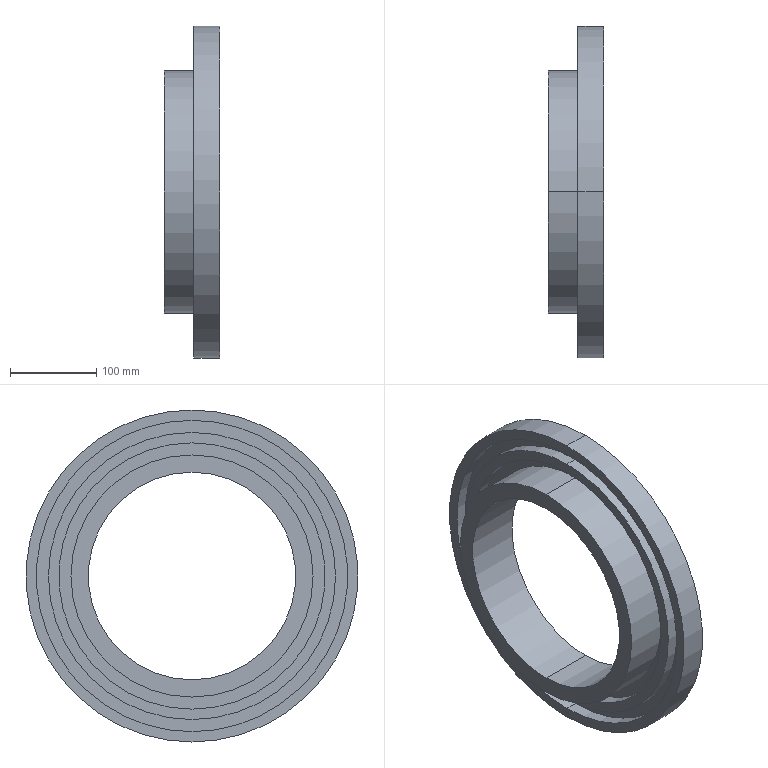Part | SolidWorks | features Revolution 1 | 1 solid | 18 faces | box 64 x 384 x 384 mm | volume 2278534 mm3 | cylinder 12 | plane 6 | commonest cylinder face diameters 240 x2 280 x2 308 x2 332 x2 360 x2 384 x2
STEP:
#1=CARTESIAN_POINT('',(64.,0.,-120.));
#2=VERTEX_POINT('',#1);
#3=CARTESIAN_POINT('',(64.,0.,120.));
#4=VERTEX_POINT('',#3);
#5=CARTESIAN_POINT('',(64.,0.,0.));
#6=DIRECTION('',(-1.,0.,0.));
#7=DIRECTION('',(0.,0.,1.));
#8=AXIS2_PLACEMENT_3D('',#5,#6,#7);
#9=CIRCLE('',#8,120.);
#10=EDGE_CURVE('',#2,#4,#9,.T.);
#11=ORIENTED_EDGE('',*,*,#10,.F.);
#12=CARTESIAN_POINT('',(0.,0.,-120.));
#13=VERTEX_POINT('',#12);
#14=CARTESIAN_POINT('',(0.,0.,-120.));
#15=DIRECTION('',(-1.,0.,0.));
#16=VECTOR('',#15,1000.);
#17=LINE('',#14,#16);
#18=EDGE_CURVE('',#2,#13,#17,.T.);
#19=ORIENTED_EDGE('',*,*,#18,.T.);
#20=CARTESIAN_POINT('',(0.,0.,120.));
#21=VERTEX_POINT('',#20);
#22=CARTESIAN_POINT('',(0.,0.,0.));
#23=DIRECTION('',(-1.,0.,0.));
#24=DIRECTION('',(0.,0.,1.));
#25=AXIS2_PLACEMENT_3D('',#22,#23,#24);
#26=CIRCLE('',#25,120.);
#27=EDGE_CURVE('',#13,#21,#26,.T.);
#28=ORIENTED_EDGE('',*,*,#27,.T.);
#29=CARTESIAN_POINT('',(0.,0.,120.));
#30=DIRECTION('',(-1.,0.,0.));
#31=VECTOR('',#30,1000.);
#32=LINE('',#29,#31);
#33=EDGE_CURVE('',#4,#21,#32,.T.);
#34=ORIENTED_EDGE('',*,*,#33,.F.);
#35=EDGE_LOOP('',(#11,#19,#28,#34));
#36=FACE_OUTER_BOUND('',#35,.T.);
#37=CARTESIAN_POINT('',(0.,0.,0.));
#38=DIRECTION('',(-1.,0.,0.));
#39=DIRECTION('',(0.,0.,1.));
#40=AXIS2_PLACEMENT_3D('',#37,#38,#39);
#41=CYLINDRICAL_SURFACE('',#40,120.);
#42=ADVANCED_FACE('',(#36),#41,.F.);
#43=CARTESIAN_POINT('',(64.,0.,192.));
#44=VERTEX_POINT('',#43);
#45=CARTESIAN_POINT('',(64.,0.,-192.));
#46=VERTEX_POINT('',#45);
#47=CARTESIAN_POINT('',(64.,0.,0.));
#48=DIRECTION('',(-1.,0.,0.));
#49=DIRECTION('',(0.,0.,1.));
#50=AXIS2_PLACEMENT_3D('',#47,#48,#49);
#51=CIRCLE('',#50,192.);
#52=EDGE_CURVE('',#44,#46,#51,.T.);
#53=ORIENTED_EDGE('',*,*,#52,.T.);
#54=CARTESIAN_POINT('',(34.,0.,-192.));
#55=VERTEX_POINT('',#54);
#56=CARTESIAN_POINT('',(0.,0.,-192.));
#57=DIRECTION('',(-1.,0.,0.));
#58=VECTOR('',#57,1000.);
#59=LINE('',#56,#58);
#60=EDGE_CURVE('',#46,#55,#59,.T.);
#61=ORIENTED_EDGE('',*,*,#60,.T.);
#62=CARTESIAN_POINT('',(34.,0.,192.));
#63=VERTEX_POINT('',#62);
#64=CARTESIAN_POINT('',(34.,0.,0.));
#65=DIRECTION('',(-1.,0.,0.));
#66=DIRECTION('',(0.,0.,1.));
#67=AXIS2_PLACEMENT_3D('',#64,#65,#66);
#68=CIRCLE('',#67,192.);
#69=EDGE_CURVE('',#63,#55,#68,.T.);
#70=ORIENTED_EDGE('',*,*,#69,.F.);
#71=CARTESIAN_POINT('',(0.,0.,192.));
#72=DIRECTION('',(-1.,0.,0.));
#73=VECTOR('',#72,1000.);
#74=LINE('',#71,#73);
#75=EDGE_CURVE('',#44,#63,#74,.T.);
#76=ORIENTED_EDGE('',*,*,#75,.F.);
#77=EDGE_LOOP('',(#53,#61,#70,#76));
#78=FACE_OUTER_BOUND('',#77,.T.);
#79=CARTESIAN_POINT('',(0.,0.,0.));
#80=DIRECTION('',(-1.,0.,0.));
#81=DIRECTION('',(0.,0.,1.));
#82=AXIS2_PLACEMENT_3D('',#79,#80,#81);
#83=CYLINDRICAL_SURFACE('',#82,192.);
#84=ADVANCED_FACE('',(#78),#83,.T.);
#85=CARTESIAN_POINT('',(48.,0.,-180.));
#86=VERTEX_POINT('',#85);
#87=CARTESIAN_POINT('',(48.,0.,180.));
#88=VERTEX_POINT('',#87);
#89=CARTESIAN_POINT('',(48.,0.,0.));
#90=DIRECTION('',(-1.,0.,0.));
#91=DIRECTION('',(0.,0.,1.));
#92=AXIS2_PLACEMENT_3D('',#89,#90,#91);
#93=CIRCLE('',#92,180.);
#94=EDGE_CURVE('',#86,#88,#93,.T.);
#95=ORIENTED_EDGE('',*,*,#94,.F.);
#96=CARTESIAN_POINT('',(34.,0.,-180.));
#97=VERTEX_POINT('',#96);
#98=CARTESIAN_POINT('',(0.,0.,-180.));
#99=DIRECTION('',(-1.,0.,0.));
#100=VECTOR('',#99,1000.);
#101=LINE('',#98,#100);
#102=EDGE_CURVE('',#86,#97,#101,.T.);
#103=ORIENTED_EDGE('',*,*,#102,.T.);
#104=CARTESIAN_POINT('',(34.,0.,180.));
#105=VERTEX_POINT('',#104);
#106=CARTESIAN_POINT('',(34.,0.,0.));
#107=DIRECTION('',(-1.,0.,0.));
#108=DIRECTION('',(0.,0.,1.));
#109=AXIS2_PLACEMENT_3D('',#106,#107,#108);
#110=CIRCLE('',#109,180.);
#111=EDGE_CURVE('',#97,#105,#110,.T.);
#112=ORIENTED_EDGE('',*,*,#111,.T.);
#113=CARTESIAN_POINT('',(0.,0.,180.));
#114=DIRECTION('',(-1.,0.,0.));
#115=VECTOR('',#114,1000.);
#116=LINE('',#113,#115);
#117=EDGE_CURVE('',#88,#105,#116,.T.);
#118=ORIENTED_EDGE('',*,*,#117,.F.);
#119=EDGE_LOOP('',(#95,#103,#112,#118));
#120=FACE_OUTER_BOUND('',#119,.T.);
#121=CARTESIAN_POINT('',(0.,0.,0.));
#122=DIRECTION('',(-1.,0.,0.));
#123=DIRECTION('',(0.,0.,1.));
#124=AXIS2_PLACEMENT_3D('',#121,#122,#123);
#125=CYLINDRICAL_SURFACE('',#124,180.);
#126=ADVANCED_FACE('',(#120),#125,.F.);
#127=CARTESIAN_POINT('',(48.,0.,166.));
#128=VERTEX_POINT('',#127);
#129=CARTESIAN_POINT('',(48.,0.,-166.));
#130=VERTEX_POINT('',#129);
#131=CARTESIAN_POINT('',(48.,0.,0.));
#132=DIRECTION('',(-1.,0.,0.));
#133=DIRECTION('',(0.,0.,1.));
#134=AXIS2_PLACEMENT_3D('',#131,#132,#133);
#135=CIRCLE('',#134,166.);
#136=EDGE_CURVE('',#128,#130,#135,.T.);
#137=ORIENTED_EDGE('',*,*,#136,.T.);
#138=CARTESIAN_POINT('',(34.,0.,-166.));
#139=VERTEX_POINT('',#138);
#140=CARTESIAN_POINT('',(0.,0.,-166.));
#141=DIRECTION('',(-1.,0.,0.));
#142=VECTOR('',#141,1000.);
#143=LINE('',#140,#142);
#144=EDGE_CURVE('',#130,#139,#143,.T.);
#145=ORIENTED_EDGE('',*,*,#144,.T.);
#146=CARTESIAN_POINT('',(34.,0.,166.));
#147=VERTEX_POINT('',#146);
#148=CARTESIAN_POINT('',(34.,0.,0.));
#149=DIRECTION('',(-1.,0.,0.));
#150=DIRECTION('',(0.,0.,1.));
#151=AXIS2_PLACEMENT_3D('',#148,#149,#150);
#152=CIRCLE('',#151,166.);
#153=EDGE_CURVE('',#147,#139,#152,.T.);
#154=ORIENTED_EDGE('',*,*,#153,.F.);
#155=CARTESIAN_POINT('',(0.,0.,166.));
#156=DIRECTION('',(-1.,0.,0.));
#157=VECTOR('',#156,1000.);
#158=LINE('',#155,#157);
#159=EDGE_CURVE('',#128,#147,#158,.T.);
#160=ORIENTED_EDGE('',*,*,#159,.F.);
#161=EDGE_LOOP('',(#137,#145,#154,#160));
#162=FACE_OUTER_BOUND('',#161,.T.);
#163=CARTESIAN_POINT('',(0.,0.,0.));
#164=DIRECTION('',(-1.,0.,0.));
#165=DIRECTION('',(0.,0.,1.));
#166=AXIS2_PLACEMENT_3D('',#163,#164,#165);
#167=CYLINDRICAL_SURFACE('',#166,166.);
#168=ADVANCED_FACE('',(#162),#167,.T.);
#169=CARTESIAN_POINT('',(48.,0.,-154.));
#170=VERTEX_POINT('',#169);
#171=CARTESIAN_POINT('',(48.,0.,154.));
#172=VERTEX_POINT('',#171);
#173=CARTESIAN_POINT('',(48.,0.,0.));
#174=DIRECTION('',(-1.,0.,0.));
#175=DIRECTION('',(0.,0.,1.));
#176=AXIS2_PLACEMENT_3D('',#173,#174,#175);
#177=CIRCLE('',#176,154.);
#178=EDGE_CURVE('',#170,#172,#177,.T.);
#179=ORIENTED_EDGE('',*,*,#178,.F.);
#180=CARTESIAN_POINT('',(34.,0.,-154.));
#181=VERTEX_POINT('',#180);
#182=CARTESIAN_POINT('',(0.,0.,-154.));
#183=DIRECTION('',(-1.,0.,0.));
#184=VECTOR('',#183,1000.);
#185=LINE('',#182,#184);
#186=EDGE_CURVE('',#170,#181,#185,.T.);
#187=ORIENTED_EDGE('',*,*,#186,.T.);
#188=CARTESIAN_POINT('',(34.,0.,154.));
#189=VERTEX_POINT('',#188);
#190=CARTESIAN_POINT('',(34.,0.,0.));
#191=DIRECTION('',(-1.,0.,0.));
#192=DIRECTION('',(0.,0.,1.));
#193=AXIS2_PLACEMENT_3D('',#190,#191,#192);
#194=CIRCLE('',#193,154.);
#195=EDGE_CURVE('',#181,#189,#194,.T.);
#196=ORIENTED_EDGE('',*,*,#195,.T.);
#197=CARTESIAN_POINT('',(0.,0.,154.));
#198=DIRECTION('',(-1.,0.,0.));
#199=VECTOR('',#198,1000.);
#200=LINE('',#197,#199);
#201=EDGE_CURVE('',#172,#189,#200,.T.);
#202=ORIENTED_EDGE('',*,*,#201,.F.);
#203=EDGE_LOOP('',(#179,#187,#196,#202));
#204=FACE_OUTER_BOUND('',#203,.T.);
#205=CARTESIAN_POINT('',(0.,0.,0.));
#206=DIRECTION('',(-1.,0.,0.));
#207=DIRECTION('',(0.,0.,1.));
#208=AXIS2_PLACEMENT_3D('',#205,#206,#207);
#209=CYLINDRICAL_SURFACE('',#208,154.);
#210=ADVANCED_FACE('',(#204),#209,.F.);
#211=CARTESIAN_POINT('',(48.,0.,140.));
#212=VERTEX_POINT('',#211);
#213=CARTESIAN_POINT('',(48.,0.,-140.));
#214=VERTEX_POINT('',#213);
#215=CARTESIAN_POINT('',(48.,0.,0.));
#216=DIRECTION('',(-1.,0.,0.));
#217=DIRECTION('',(0.,0.,1.));
#218=AXIS2_PLACEMENT_3D('',#215,#216,#217);
#219=CIRCLE('',#218,140.);
#220=EDGE_CURVE('',#212,#214,#219,.T.);
#221=ORIENTED_EDGE('',*,*,#220,.T.);
#222=CARTESIAN_POINT('',(0.,0.,-140.));
#223=VERTEX_POINT('',#222);
#224=CARTESIAN_POINT('',(0.,0.,-140.));
#225=DIRECTION('',(-1.,0.,0.));
#226=VECTOR('',#225,1000.);
#227=LINE('',#224,#226);
#228=EDGE_CURVE('',#214,#223,#227,.T.);
#229=ORIENTED_EDGE('',*,*,#228,.T.);
#230=CARTESIAN_POINT('',(0.,0.,140.));
#231=VERTEX_POINT('',#230);
#232=CARTESIAN_POINT('',(0.,0.,0.));
#233=DIRECTION('',(-1.,0.,0.));
#234=DIRECTION('',(0.,0.,1.));
#235=AXIS2_PLACEMENT_3D('',#232,#233,#234);
#236=CIRCLE('',#235,140.);
#237=EDGE_CURVE('',#231,#223,#236,.T.);
#238=ORIENTED_EDGE('',*,*,#237,.F.);
#239=CARTESIAN_POINT('',(0.,0.,140.));
#240=DIRECTION('',(-1.,0.,0.));
#241=VECTOR('',#240,1000.);
#242=LINE('',#239,#241);
#243=EDGE_CURVE('',#212,#231,#242,.T.);
#244=ORIENTED_EDGE('',*,*,#243,.F.);
#245=EDGE_LOOP('',(#221,#229,#238,#244));
#246=FACE_OUTER_BOUND('',#245,.T.);
#247=CARTESIAN_POINT('',(0.,0.,0.));
#248=DIRECTION('',(-1.,0.,0.));
#249=DIRECTION('',(0.,0.,1.));
#250=AXIS2_PLACEMENT_3D('',#247,#248,#249);
#251=CYLINDRICAL_SURFACE('',#250,140.);
#252=ADVANCED_FACE('',(#246),#251,.T.);
#253=ORIENTED_EDGE('',*,*,#228,.F.);
#254=CARTESIAN_POINT('',(48.,0.,0.));
#255=DIRECTION('',(-1.,0.,0.));
#256=DIRECTION('',(0.,0.,1.));
#257=AXIS2_PLACEMENT_3D('',#254,#255,#256);
#258=CIRCLE('',#257,140.);
#259=EDGE_CURVE('',#214,#212,#258,.T.);
#260=ORIENTED_EDGE('',*,*,#259,.T.);
#261=ORIENTED_EDGE('',*,*,#243,.T.);
#262=CARTESIAN_POINT('',(0.,0.,0.));
#263=DIRECTION('',(-1.,0.,0.));
#264=DIRECTION('',(0.,0.,1.));
#265=AXIS2_PLACEMENT_3D('',#262,#263,#264);
#266=CIRCLE('',#265,140.);
#267=EDGE_CURVE('',#223,#231,#266,.T.);
#268=ORIENTED_EDGE('',*,*,#267,.F.);
#269=EDGE_LOOP('',(#253,#260,#261,#268));
#270=FACE_OUTER_BOUND('',#269,.T.);
#271=CARTESIAN_POINT('',(0.,0.,0.));
#272=DIRECTION('',(-1.,0.,0.));
#273=DIRECTION('',(0.,0.,1.));
#274=AXIS2_PLACEMENT_3D('',#271,#272,#273);
#275=CYLINDRICAL_SURFACE('',#274,140.);
#276=ADVANCED_FACE('',(#270),#275,.T.);
#277=ORIENTED_EDGE('',*,*,#220,.F.);
#278=ORIENTED_EDGE('',*,*,#259,.F.);
#279=EDGE_LOOP('',(#277,#278));
#280=FACE_BOUND('',#279,.T.);
#281=CARTESIAN_POINT('',(48.,0.,0.));
#282=DIRECTION('',(-1.,0.,0.));
#283=DIRECTION('',(0.,0.,1.));
#284=AXIS2_PLACEMENT_3D('',#281,#282,#283);
#285=CIRCLE('',#284,154.);
#286=EDGE_CURVE('',#172,#170,#285,.T.);
#287=ORIENTED_EDGE('',*,*,#286,.T.);
#288=ORIENTED_EDGE('',*,*,#178,.T.);
#289=EDGE_LOOP('',(#287,#288));
#290=FACE_OUTER_BOUND('',#289,.T.);
#291=CARTESIAN_POINT('',(48.,154.,0.));
#292=DIRECTION('',(1.,0.,0.));
#293=DIRECTION('',(0.,0.,-1.));
#294=AXIS2_PLACEMENT_3D('',#291,#292,#293);
#295=PLANE('',#294);
#296=ADVANCED_FACE('',(#280,#290),#295,.F.);
#297=ORIENTED_EDGE('',*,*,#186,.F.);
#298=ORIENTED_EDGE('',*,*,#286,.F.);
#299=ORIENTED_EDGE('',*,*,#201,.T.);
#300=CARTESIAN_POINT('',(34.,0.,0.));
#301=DIRECTION('',(-1.,0.,0.));
#302=DIRECTION('',(0.,0.,1.));
#303=AXIS2_PLACEMENT_3D('',#300,#301,#302);
#304=CIRCLE('',#303,154.);
#305=EDGE_CURVE('',#189,#181,#304,.T.);
#306=ORIENTED_EDGE('',*,*,#305,.T.);
#307=EDGE_LOOP('',(#297,#298,#299,#306));
#308=FACE_OUTER_BOUND('',#307,.T.);
#309=CARTESIAN_POINT('',(0.,0.,0.));
#310=DIRECTION('',(-1.,0.,0.));
#311=DIRECTION('',(0.,0.,1.));
#312=AXIS2_PLACEMENT_3D('',#309,#310,#311);
#313=CYLINDRICAL_SURFACE('',#312,154.);
#314=ADVANCED_FACE('',(#308),#313,.F.);
#315=ORIENTED_EDGE('',*,*,#305,.F.);
#316=ORIENTED_EDGE('',*,*,#195,.F.);
#317=EDGE_LOOP('',(#315,#316));
#318=FACE_BOUND('',#317,.T.);
#319=ORIENTED_EDGE('',*,*,#153,.T.);
#320=CARTESIAN_POINT('',(34.,0.,0.));
#321=DIRECTION('',(-1.,0.,0.));
#322=DIRECTION('',(0.,0.,1.));
#323=AXIS2_PLACEMENT_3D('',#320,#321,#322);
#324=CIRCLE('',#323,166.);
#325=EDGE_CURVE('',#139,#147,#324,.T.);
#326=ORIENTED_EDGE('',*,*,#325,.T.);
#327=EDGE_LOOP('',(#319,#326));
#328=FACE_OUTER_BOUND('',#327,.T.);
#329=CARTESIAN_POINT('',(34.,154.,0.));
#330=DIRECTION('',(1.,0.,0.));
#331=DIRECTION('',(0.,0.,-1.));
#332=AXIS2_PLACEMENT_3D('',#329,#330,#331);
#333=PLANE('',#332);
#334=ADVANCED_FACE('',(#318,#328),#333,.F.);
#335=ORIENTED_EDGE('',*,*,#144,.F.);
#336=CARTESIAN_POINT('',(48.,0.,0.));
#337=DIRECTION('',(-1.,0.,0.));
#338=DIRECTION('',(0.,0.,1.));
#339=AXIS2_PLACEMENT_3D('',#336,#337,#338);
#340=CIRCLE('',#339,166.);
#341=EDGE_CURVE('',#130,#128,#340,.T.);
#342=ORIENTED_EDGE('',*,*,#341,.T.);
#343=ORIENTED_EDGE('',*,*,#159,.T.);
#344=ORIENTED_EDGE('',*,*,#325,.F.);
#345=EDGE_LOOP('',(#335,#342,#343,#344));
#346=FACE_OUTER_BOUND('',#345,.T.);
#347=CARTESIAN_POINT('',(0.,0.,0.));
#348=DIRECTION('',(-1.,0.,0.));
#349=DIRECTION('',(0.,0.,1.));
#350=AXIS2_PLACEMENT_3D('',#347,#348,#349);
#351=CYLINDRICAL_SURFACE('',#350,166.);
#352=ADVANCED_FACE('',(#346),#351,.T.);
#353=ORIENTED_EDGE('',*,*,#136,.F.);
#354=ORIENTED_EDGE('',*,*,#341,.F.);
#355=EDGE_LOOP('',(#353,#354));
#356=FACE_BOUND('',#355,.T.);
#357=CARTESIAN_POINT('',(48.,0.,0.));
#358=DIRECTION('',(-1.,0.,0.));
#359=DIRECTION('',(0.,0.,1.));
#360=AXIS2_PLACEMENT_3D('',#357,#358,#359);
#361=CIRCLE('',#360,180.);
#362=EDGE_CURVE('',#88,#86,#361,.T.);
#363=ORIENTED_EDGE('',*,*,#362,.T.);
#364=ORIENTED_EDGE('',*,*,#94,.T.);
#365=EDGE_LOOP('',(#363,#364));
#366=FACE_OUTER_BOUND('',#365,.T.);
#367=CARTESIAN_POINT('',(48.,180.,0.));
#368=DIRECTION('',(1.,0.,0.));
#369=DIRECTION('',(0.,0.,-1.));
#370=AXIS2_PLACEMENT_3D('',#367,#368,#369);
#371=PLANE('',#370);
#372=ADVANCED_FACE('',(#356,#366),#371,.F.);
#373=ORIENTED_EDGE('',*,*,#102,.F.);
#374=ORIENTED_EDGE('',*,*,#362,.F.);
#375=ORIENTED_EDGE('',*,*,#117,.T.);
#376=CARTESIAN_POINT('',(34.,0.,0.));
#377=DIRECTION('',(-1.,0.,0.));
#378=DIRECTION('',(0.,0.,1.));
#379=AXIS2_PLACEMENT_3D('',#376,#377,#378);
#380=CIRCLE('',#379,180.);
#381=EDGE_CURVE('',#105,#97,#380,.T.);
#382=ORIENTED_EDGE('',*,*,#381,.T.);
#383=EDGE_LOOP('',(#373,#374,#375,#382));
#384=FACE_OUTER_BOUND('',#383,.T.);
#385=CARTESIAN_POINT('',(0.,0.,0.));
#386=DIRECTION('',(-1.,0.,0.));
#387=DIRECTION('',(0.,0.,1.));
#388=AXIS2_PLACEMENT_3D('',#385,#386,#387);
#389=CYLINDRICAL_SURFACE('',#388,180.);
#390=ADVANCED_FACE('',(#384),#389,.F.);
#391=ORIENTED_EDGE('',*,*,#381,.F.);
#392=ORIENTED_EDGE('',*,*,#111,.F.);
#393=EDGE_LOOP('',(#391,#392));
#394=FACE_BOUND('',#393,.T.);
#395=ORIENTED_EDGE('',*,*,#69,.T.);
#396=CARTESIAN_POINT('',(34.,0.,0.));
#397=DIRECTION('',(-1.,0.,0.));
#398=DIRECTION('',(0.,0.,1.));
#399=AXIS2_PLACEMENT_3D('',#396,#397,#398);
#400=CIRCLE('',#399,192.);
#401=EDGE_CURVE('',#55,#63,#400,.T.);
#402=ORIENTED_EDGE('',*,*,#401,.T.);
#403=EDGE_LOOP('',(#395,#402));
#404=FACE_OUTER_BOUND('',#403,.T.);
#405=CARTESIAN_POINT('',(34.,180.,0.));
#406=DIRECTION('',(1.,0.,0.));
#407=DIRECTION('',(0.,0.,-1.));
#408=AXIS2_PLACEMENT_3D('',#405,#406,#407);
#409=PLANE('',#408);
#410=ADVANCED_FACE('',(#394,#404),#409,.F.);
#411=ORIENTED_EDGE('',*,*,#60,.F.);
#412=CARTESIAN_POINT('',(64.,0.,0.));
#413=DIRECTION('',(-1.,0.,0.));
#414=DIRECTION('',(0.,0.,1.));
#415=AXIS2_PLACEMENT_3D('',#412,#413,#414);
#416=CIRCLE('',#415,192.);
#417=EDGE_CURVE('',#46,#44,#416,.T.);
#418=ORIENTED_EDGE('',*,*,#417,.T.);
#419=ORIENTED_EDGE('',*,*,#75,.T.);
#420=ORIENTED_EDGE('',*,*,#401,.F.);
#421=EDGE_LOOP('',(#411,#418,#419,#420));
#422=FACE_OUTER_BOUND('',#421,.T.);
#423=CARTESIAN_POINT('',(0.,0.,0.));
#424=DIRECTION('',(-1.,0.,0.));
#425=DIRECTION('',(0.,0.,1.));
#426=AXIS2_PLACEMENT_3D('',#423,#424,#425);
#427=CYLINDRICAL_SURFACE('',#426,192.);
#428=ADVANCED_FACE('',(#422),#427,.T.);
#429=ORIENTED_EDGE('',*,*,#52,.F.);
#430=ORIENTED_EDGE('',*,*,#417,.F.);
#431=EDGE_LOOP('',(#429,#430));
#432=FACE_OUTER_BOUND('',#431,.T.);
#433=CARTESIAN_POINT('',(64.,0.,0.));
#434=DIRECTION('',(-1.,0.,0.));
#435=DIRECTION('',(0.,0.,1.));
#436=AXIS2_PLACEMENT_3D('',#433,#434,#435);
#437=CIRCLE('',#436,120.);
#438=EDGE_CURVE('',#4,#2,#437,.T.);
#439=ORIENTED_EDGE('',*,*,#438,.T.);
#440=ORIENTED_EDGE('',*,*,#10,.T.);
#441=EDGE_LOOP('',(#439,#440));
#442=FACE_BOUND('',#441,.T.);
#443=CARTESIAN_POINT('',(64.,192.,0.));
#444=DIRECTION('',(-1.,0.,0.));
#445=DIRECTION('',(0.,0.,1.));
#446=AXIS2_PLACEMENT_3D('',#443,#444,#445);
#447=PLANE('',#446);
#448=ADVANCED_FACE('',(#432,#442),#447,.F.);
#449=ORIENTED_EDGE('',*,*,#18,.F.);
#450=ORIENTED_EDGE('',*,*,#438,.F.);
#451=ORIENTED_EDGE('',*,*,#33,.T.);
#452=CARTESIAN_POINT('',(0.,0.,0.));
#453=DIRECTION('',(-1.,0.,0.));
#454=DIRECTION('',(0.,0.,1.));
#455=AXIS2_PLACEMENT_3D('',#452,#453,#454);
#456=CIRCLE('',#455,120.);
#457=EDGE_CURVE('',#21,#13,#456,.T.);
#458=ORIENTED_EDGE('',*,*,#457,.T.);
#459=EDGE_LOOP('',(#449,#450,#451,#458));
#460=FACE_OUTER_BOUND('',#459,.T.);
#461=CARTESIAN_POINT('',(0.,0.,0.));
#462=DIRECTION('',(-1.,0.,0.));
#463=DIRECTION('',(0.,0.,1.));
#464=AXIS2_PLACEMENT_3D('',#461,#462,#463);
#465=CYLINDRICAL_SURFACE('',#464,120.);
#466=ADVANCED_FACE('',(#460),#465,.F.);
#467=ORIENTED_EDGE('',*,*,#457,.F.);
#468=ORIENTED_EDGE('',*,*,#27,.F.);
#469=EDGE_LOOP('',(#467,#468));
#470=FACE_BOUND('',#469,.T.);
#471=ORIENTED_EDGE('',*,*,#237,.T.);
#472=ORIENTED_EDGE('',*,*,#267,.T.);
#473=EDGE_LOOP('',(#471,#472));
#474=FACE_OUTER_BOUND('',#473,.T.);
#475=CARTESIAN_POINT('',(0.,120.,0.));
#476=DIRECTION('',(1.,0.,0.));
#477=DIRECTION('',(0.,0.,-1.));
#478=AXIS2_PLACEMENT_3D('',#475,#476,#477);
#479=PLANE('',#478);
#480=ADVANCED_FACE('',(#470,#474),#479,.F.);
#481=CLOSED_SHELL('',(#42,#84,#126,#168,#210,#252,#276,#296,#314,#334,#352,#372,#390,#410,#428,#448,#466,#480));
#482=MANIFOLD_SOLID_BREP('',#481);
#483=CARTESIAN_POINT('',(0.,0.,0.));
#484=DIRECTION('',(0.,0.,1.));
#485=DIRECTION('',(1.,0.,0.));
#486=AXIS2_PLACEMENT_3D('',#483,#484,#485);
#487=(LENGTH_UNIT()NAMED_UNIT(*)SI_UNIT(.MILLI.,.METRE.));
#488=UNCERTAINTY_MEASURE_WITH_UNIT(LENGTH_MEASURE(0.00001),#487,'','');
#489=(NAMED_UNIT(*)PLANE_ANGLE_UNIT()SI_UNIT($,.RADIAN.));
#490=(NAMED_UNIT(*)SI_UNIT($,.STERADIAN.)SOLID_ANGLE_UNIT());
#491=(GEOMETRIC_REPRESENTATION_CONTEXT(3)GLOBAL_UNCERTAINTY_ASSIGNED_CONTEXT((#488))GLOBAL_UNIT_ASSIGNED_CONTEXT((#487,#489,#490))REPRESENTATION_CONTEXT('',''));
#492=ADVANCED_BREP_SHAPE_REPRESENTATION('',(#482,#486),#491);